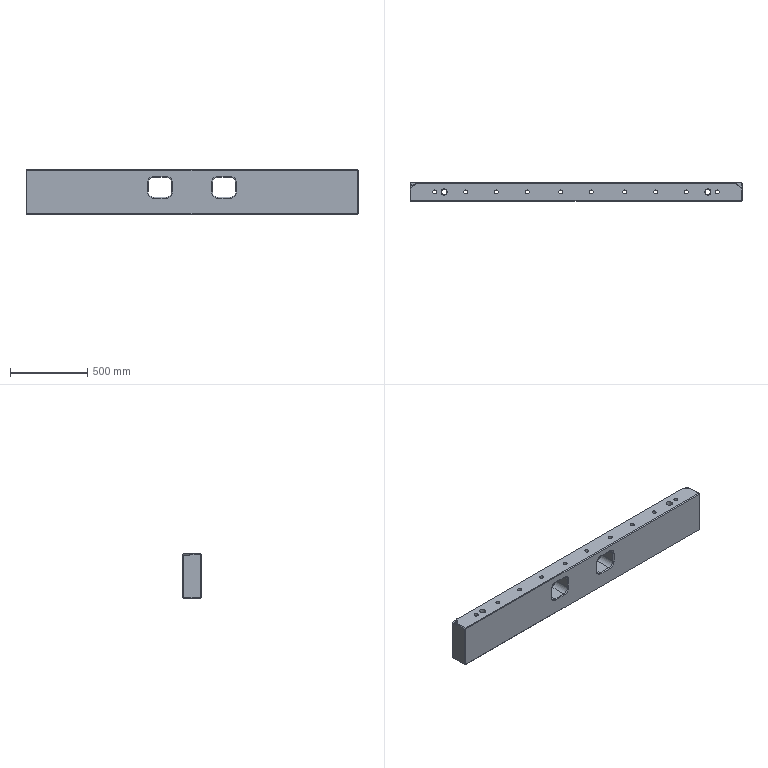Part | STEP file | solid 229 | 1 solid | 181 faces | box 2150 x 120 x 290 mm | volume 67733928 mm3 | plane 72 | cylinder 67 | cone 26 | torus 16 | commonest cylinder face diameters 12 x16 21 x11 26 x10 39 x10 70 x8 5 x6